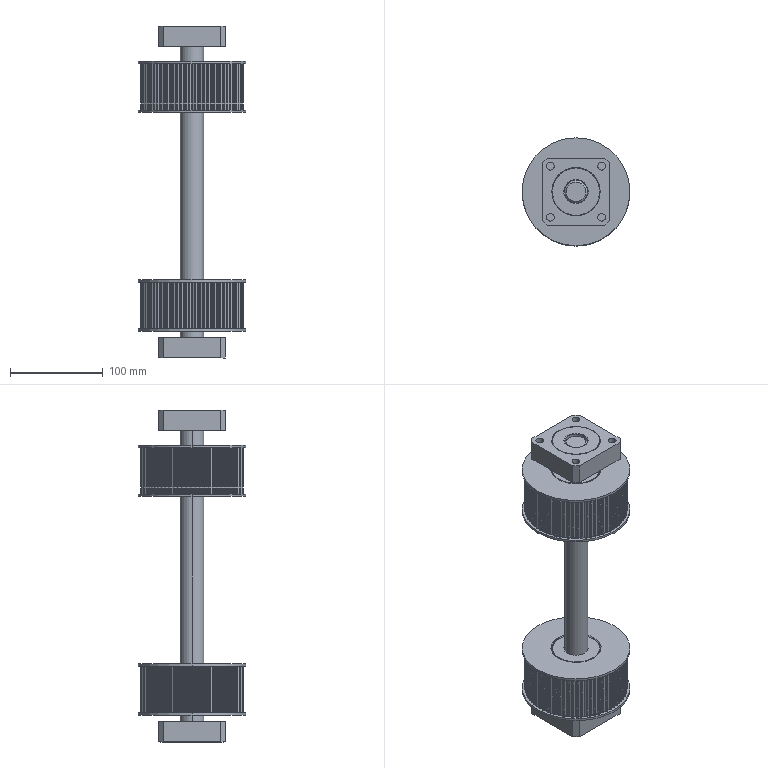Part | 11 solids | 854 faces | box 116 x 116 x 357 mm | volume 1318520 mm3 | cylinder 732 | cone 68 | plane 54 | commonest cylinder face diameters 2.5 x508 110 x142 52 x24 25 x18 8.5 x16 13 x16